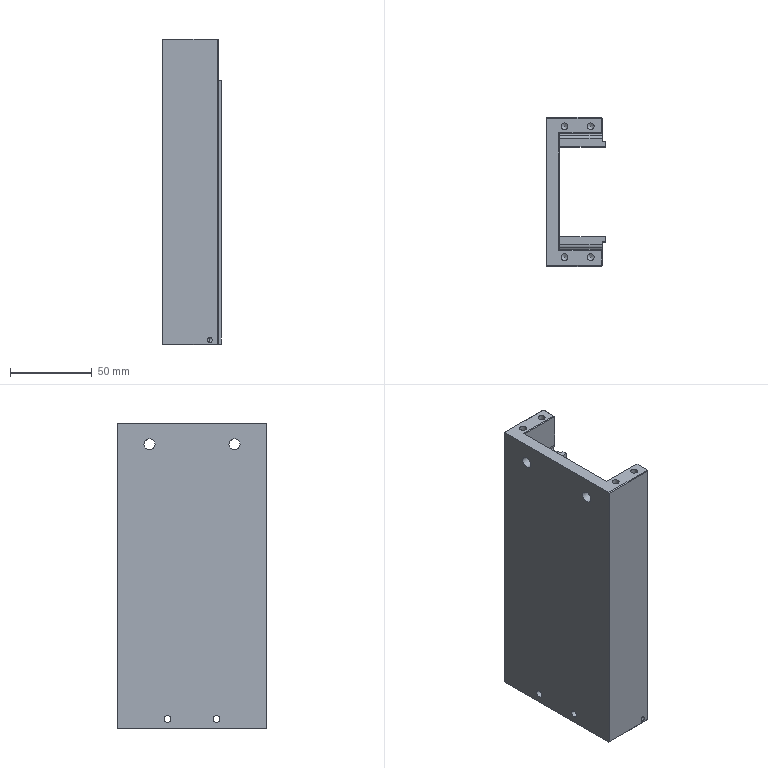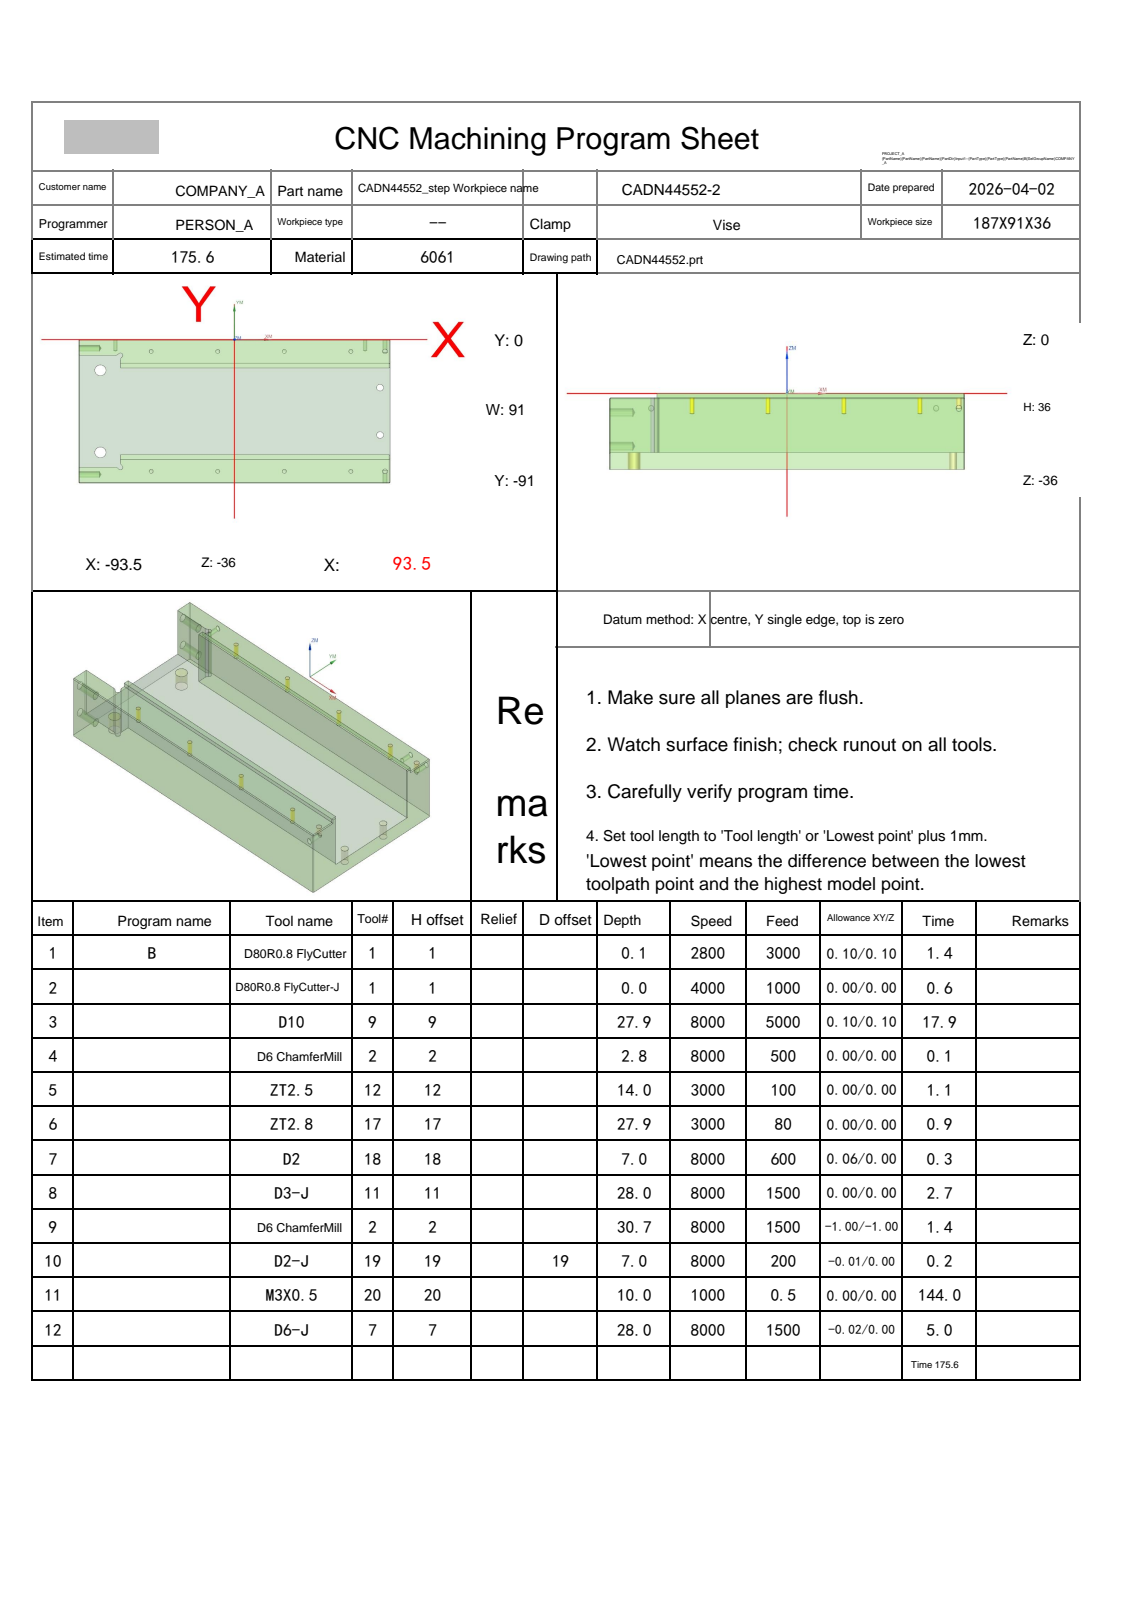NC program | NX | posted by the shop | part box 36 x 91 x 187 mm
Lines 1 to 127 of 12140:
%
O0001
(Machine time: 305.95 MIN)
(===Total Tool:10===)
(T1=D80R0.8 FlyCutter D=80.  R=0.8  D-  H01 Z=-0.   )
(T9=D10     D=10.  R=0.   D-  H09 Z=-27.9 )
(T2=D6 ChamferMill   D=6.   R=0.   D-  H02 Z=-30.7 )
(T12=ZT2.5  D=2.5  DR_a=118 D-  H12 Z=-14.  )
(T17=ZT2.8  D=2.8  DR_a=118 D-  H17 Z=-27.9 )
(T18=D2     D=2.   R=0.   D-  H18 Z=-7.   )
(T11=D3-J   D=2.95 R=0.   D-  H11 Z=-28.  )
(T19=D2-J   D=2.   R=0.   D19 H19 Z=-7.   )
(T20=M3X0.5 D=2.5  DR_a=180 D-  H20 Z=-10.  )
(T7=D6-J    D=6.   R=0.   D7  H07 Z=-28.  )
G80 G90 G17 G49 G40
G91 G28 Z0
M01
N1 T01 M06
(D80R0.8 FlyCutter  D=80. R=0.8 H=01 ce=0.10 di=0.10)
G00 G90 G54 X-145.597 Y-23.903 M03 S2800
G43 H01 Z20.
M08
Z5.014
G01 Z3.014 F3000.
X-133.597
X126.397
G02 X133.597 Y-31.103 I0.0 J-7.2
G01 Y-51.737
G02 X125.597 Y-59.737 I-8. J0.0
G01 X-133.597
X-145.597
Z5.014
G00 Y-23.903
Z4.529
G01 Z2.529
X-133.597
X126.397
G02 X133.597 Y-31.103 I0.0 J-7.2
G01 Y-51.737
G02 X125.597 Y-59.737 I-8. J0.0
G01 X-133.597
X-145.597
Z4.529
G00 Y-23.903
Z4.043
G01 Z2.043
X-133.597
X126.397
G02 X133.597 Y-31.103 I0.0 J-7.2
G01 Y-51.737
G02 X125.597 Y-59.737 I-8. J0.0
G01 X-133.597
X-145.597
Z4.043
G00 Y-23.903
Z3.557
G01 Z1.557
X-133.597
X126.397
G02 X133.597 Y-31.103 I0.0 J-7.2
G01 Y-51.737
G02 X125.597 Y-59.737 I-8. J0.0
G01 X-133.597
X-145.597
Z3.557
G00 Y-23.903
Z3.071
G01 Z1.071
X-133.597
X126.397
G02 X133.597 Y-31.103 I0.0 J-7.2
G01 Y-51.737
G02 X125.597 Y-59.737 I-8. J0.0
G01 X-133.597
X-145.597
Z3.071
G00 Y-23.903
Z2.586
G01 Z.586
X-133.597
X126.397
G02 X133.597 Y-31.103 I0.0 J-7.2
G01 Y-51.737
G02 X125.597 Y-59.737 I-8. J0.0
G01 X-133.597
X-145.597
Z2.586
G00 Y-23.903
Z2.1
G01 Z.1
X-133.597
X126.397
G02 X133.597 Y-31.103 I0.0 J-7.2
G01 Y-51.737
G02 X125.597 Y-59.737 I-8. J0.0
G01 X-133.597
X-145.597
Z2.1
G00 Z20.
G91 G28 Z0.0
M05
M09
G91 G28 Z0.0
M01
N2 T01 M06
(D80R0.8 FlyCutter-J  D=80. R=0.8 H=01 ce=0.00 di=0.00)
G00 G90 G54 X-145.499 Y-24.001 M03 S4000
G43 H01 Z20.
M08
Z2.
G01 Z0.0 F1000.
X-133.499
X126.299
G02 X133.499 Y-31.201 I0.0 J-7.2
G01 Y-51.639
G02 X125.499 Y-59.639 I-8. J0.0
G01 X-133.499
X-145.499
Z2.
G00 Z20.
G91 G28 Z0.0
M05
M09
G91 G28 Z0.0
M01